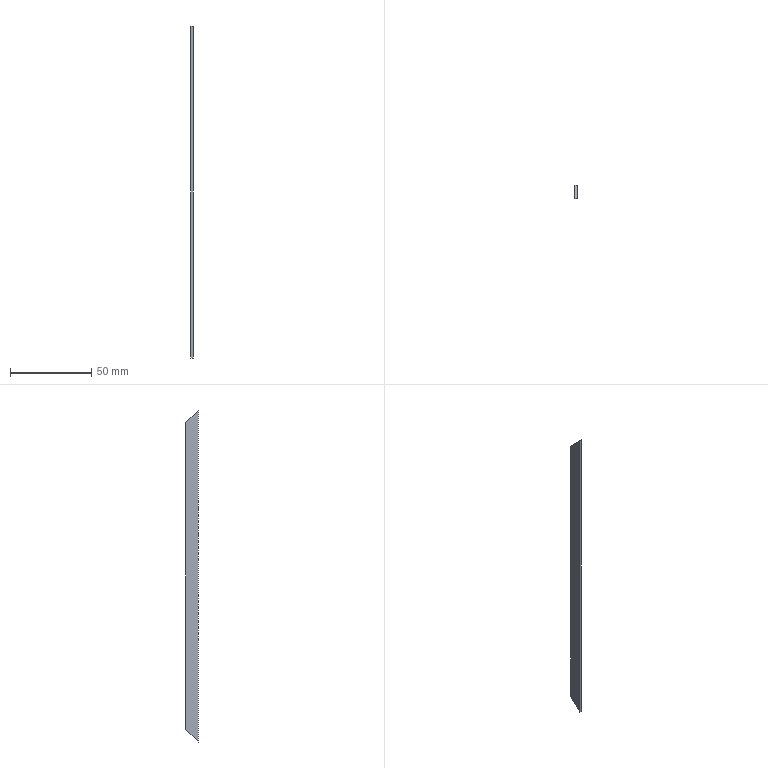Part | NX | features BREP 1 | 1 solid | 6 faces | box 1.5 x 8 x 204.5 mm | volume 2358 mm3 | plane 6
STEP:
#1=CARTESIAN_POINT('',(0.,8.,94.25));
#2=VERTEX_POINT('',#1);
#3=CARTESIAN_POINT('',(0.,8.,-94.25));
#4=VERTEX_POINT('',#3);
#5=CARTESIAN_POINT('',(0.,8.,102.25));
#6=DIRECTION('',(0.,0.,-1.));
#7=VECTOR('',#6,1000.);
#8=LINE('',#5,#7);
#9=EDGE_CURVE('',#2,#4,#8,.T.);
#10=ORIENTED_EDGE('',*,*,#9,.T.);
#11=CARTESIAN_POINT('',(0.,0.,-102.25));
#12=VERTEX_POINT('',#11);
#13=CARTESIAN_POINT('',(0.,8.,-94.25));
#14=DIRECTION('',(0.,-0.7071,-0.7071));
#15=VECTOR('',#14,1000.);
#16=LINE('',#13,#15);
#17=EDGE_CURVE('',#4,#12,#16,.T.);
#18=ORIENTED_EDGE('',*,*,#17,.T.);
#19=CARTESIAN_POINT('',(0.,0.,102.25));
#20=VERTEX_POINT('',#19);
#21=CARTESIAN_POINT('',(0.,0.,102.25));
#22=DIRECTION('',(0.,0.,-1.));
#23=VECTOR('',#22,1000.);
#24=LINE('',#21,#23);
#25=EDGE_CURVE('',#20,#12,#24,.T.);
#26=ORIENTED_EDGE('',*,*,#25,.F.);
#27=CARTESIAN_POINT('',(0.,0.,102.25));
#28=DIRECTION('',(0.,0.7071,-0.7071));
#29=VECTOR('',#28,1000.);
#30=LINE('',#27,#29);
#31=EDGE_CURVE('',#20,#2,#30,.T.);
#32=ORIENTED_EDGE('',*,*,#31,.T.);
#33=EDGE_LOOP('',(#10,#18,#26,#32));
#34=FACE_BOUND('',#33,.T.);
#35=CARTESIAN_POINT('',(0.,0.,102.25));
#36=DIRECTION('',(1.,0.,0.));
#37=DIRECTION('',(0.,1.,0.));
#38=AXIS2_PLACEMENT_3D('',#35,#36,#37);
#39=PLANE('',#38);
#40=ADVANCED_FACE('',(#34),#39,.F.);
#41=CARTESIAN_POINT('',(1.5,0.,-102.25));
#42=VERTEX_POINT('',#41);
#43=CARTESIAN_POINT('',(0.,0.,-102.25));
#44=DIRECTION('',(1.,0.,0.));
#45=VECTOR('',#44,1000.);
#46=LINE('',#43,#45);
#47=EDGE_CURVE('',#12,#42,#46,.T.);
#48=ORIENTED_EDGE('',*,*,#47,.T.);
#49=CARTESIAN_POINT('',(1.5,0.,102.25));
#50=VERTEX_POINT('',#49);
#51=CARTESIAN_POINT('',(1.5,0.,102.25));
#52=DIRECTION('',(0.,0.,-1.));
#53=VECTOR('',#52,1000.);
#54=LINE('',#51,#53);
#55=EDGE_CURVE('',#50,#42,#54,.T.);
#56=ORIENTED_EDGE('',*,*,#55,.F.);
#57=CARTESIAN_POINT('',(0.,0.,102.25));
#58=DIRECTION('',(1.,0.,0.));
#59=VECTOR('',#58,1000.);
#60=LINE('',#57,#59);
#61=EDGE_CURVE('',#20,#50,#60,.T.);
#62=ORIENTED_EDGE('',*,*,#61,.F.);
#63=ORIENTED_EDGE('',*,*,#25,.T.);
#64=EDGE_LOOP('',(#48,#56,#62,#63));
#65=FACE_BOUND('',#64,.T.);
#66=CARTESIAN_POINT('',(0.,0.,102.25));
#67=DIRECTION('',(0.,1.,0.));
#68=DIRECTION('',(1.,0.,0.));
#69=AXIS2_PLACEMENT_3D('',#66,#67,#68);
#70=PLANE('',#69);
#71=ADVANCED_FACE('',(#65),#70,.F.);
#72=ORIENTED_EDGE('',*,*,#55,.T.);
#73=CARTESIAN_POINT('',(1.5,8.,-94.25));
#74=VERTEX_POINT('',#73);
#75=CARTESIAN_POINT('',(1.5,8.,-94.25));
#76=DIRECTION('',(0.,0.7071,0.7071));
#77=VECTOR('',#76,1000.);
#78=LINE('',#75,#77);
#79=EDGE_CURVE('',#42,#74,#78,.T.);
#80=ORIENTED_EDGE('',*,*,#79,.T.);
#81=CARTESIAN_POINT('',(1.5,8.,94.25));
#82=VERTEX_POINT('',#81);
#83=CARTESIAN_POINT('',(1.5,8.,102.25));
#84=DIRECTION('',(0.,0.,-1.));
#85=VECTOR('',#84,1000.);
#86=LINE('',#83,#85);
#87=EDGE_CURVE('',#82,#74,#86,.T.);
#88=ORIENTED_EDGE('',*,*,#87,.F.);
#89=CARTESIAN_POINT('',(1.5,0.,102.25));
#90=DIRECTION('',(0.,-0.7071,0.7071));
#91=VECTOR('',#90,1000.);
#92=LINE('',#89,#91);
#93=EDGE_CURVE('',#82,#50,#92,.T.);
#94=ORIENTED_EDGE('',*,*,#93,.T.);
#95=EDGE_LOOP('',(#72,#80,#88,#94));
#96=FACE_BOUND('',#95,.T.);
#97=CARTESIAN_POINT('',(1.5,0.,102.25));
#98=DIRECTION('',(-1.,0.,0.));
#99=DIRECTION('',(0.,0.,1.));
#100=AXIS2_PLACEMENT_3D('',#97,#98,#99);
#101=PLANE('',#100);
#102=ADVANCED_FACE('',(#96),#101,.F.);
#103=ORIENTED_EDGE('',*,*,#87,.T.);
#104=CARTESIAN_POINT('',(0.,8.,-94.25));
#105=DIRECTION('',(-1.,0.,0.));
#106=VECTOR('',#105,1000.);
#107=LINE('',#104,#106);
#108=EDGE_CURVE('',#74,#4,#107,.T.);
#109=ORIENTED_EDGE('',*,*,#108,.T.);
#110=ORIENTED_EDGE('',*,*,#9,.F.);
#111=CARTESIAN_POINT('',(0.,8.,94.25));
#112=DIRECTION('',(1.,0.,0.));
#113=VECTOR('',#112,1000.);
#114=LINE('',#111,#113);
#115=EDGE_CURVE('',#2,#82,#114,.T.);
#116=ORIENTED_EDGE('',*,*,#115,.T.);
#117=EDGE_LOOP('',(#103,#109,#110,#116));
#118=FACE_BOUND('',#117,.T.);
#119=CARTESIAN_POINT('',(0.,8.,102.25));
#120=DIRECTION('',(0.,-1.,0.));
#121=DIRECTION('',(0.,0.,-1.));
#122=AXIS2_PLACEMENT_3D('',#119,#120,#121);
#123=PLANE('',#122);
#124=ADVANCED_FACE('',(#118),#123,.F.);
#125=ORIENTED_EDGE('',*,*,#79,.F.);
#126=ORIENTED_EDGE('',*,*,#47,.F.);
#127=ORIENTED_EDGE('',*,*,#17,.F.);
#128=ORIENTED_EDGE('',*,*,#108,.F.);
#129=EDGE_LOOP('',(#125,#126,#127,#128));
#130=FACE_BOUND('',#129,.T.);
#131=CARTESIAN_POINT('',(0.,8.,-94.25));
#132=DIRECTION('',(0.,0.7071,-0.7071));
#133=DIRECTION('',(-1.,0.,0.));
#134=AXIS2_PLACEMENT_3D('',#131,#132,#133);
#135=PLANE('',#134);
#136=ADVANCED_FACE('',(#130),#135,.T.);
#137=ORIENTED_EDGE('',*,*,#93,.F.);
#138=ORIENTED_EDGE('',*,*,#115,.F.);
#139=ORIENTED_EDGE('',*,*,#31,.F.);
#140=ORIENTED_EDGE('',*,*,#61,.T.);
#141=EDGE_LOOP('',(#137,#138,#139,#140));
#142=FACE_BOUND('',#141,.T.);
#143=CARTESIAN_POINT('',(0.,0.,102.25));
#144=DIRECTION('',(0.,-0.7071,-0.7071));
#145=DIRECTION('',(0.,0.7071,-0.7071));
#146=AXIS2_PLACEMENT_3D('',#143,#144,#145);
#147=PLANE('',#146);
#148=ADVANCED_FACE('',(#142),#147,.F.);
#149=CLOSED_SHELL('',(#40,#71,#102,#124,#136,#148));
#150=MANIFOLD_SOLID_BREP('',#149);
#151=(LENGTH_UNIT()NAMED_UNIT(*)SI_UNIT(.MILLI.,.METRE.));
#152=UNCERTAINTY_MEASURE_WITH_UNIT(LENGTH_MEASURE(0.00001),#151,'','');
#153=(NAMED_UNIT(*)PLANE_ANGLE_UNIT()SI_UNIT($,.RADIAN.));
#154=(NAMED_UNIT(*)SI_UNIT($,.STERADIAN.)SOLID_ANGLE_UNIT());
#155=(GEOMETRIC_REPRESENTATION_CONTEXT(3)GLOBAL_UNCERTAINTY_ASSIGNED_CONTEXT((#152))GLOBAL_UNIT_ASSIGNED_CONTEXT((#151,#153,#154))REPRESENTATION_CONTEXT('',''));
#156=ADVANCED_BREP_SHAPE_REPRESENTATION('',(#150),#155);